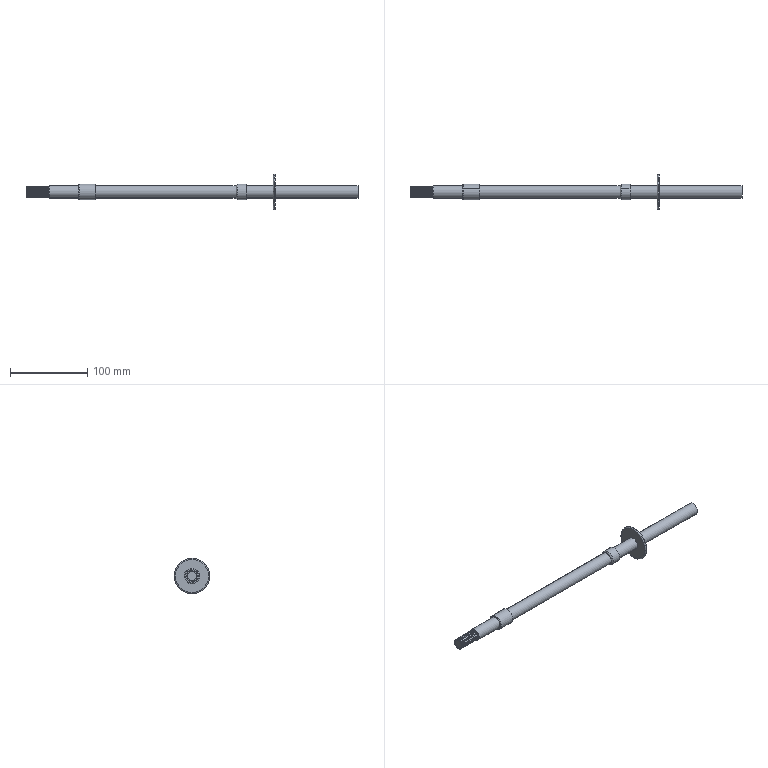Part | SolidWorks | features MBimport 1 | 1 solid | 86 faces | box 430 x 46 x 46 mm | volume 92426 mm3 | cylinder 43 | plane 33 | cone 6 | torus 4 | commonest cylinder face diameters 14 x13 11.172 x12 16 x12 20 x6